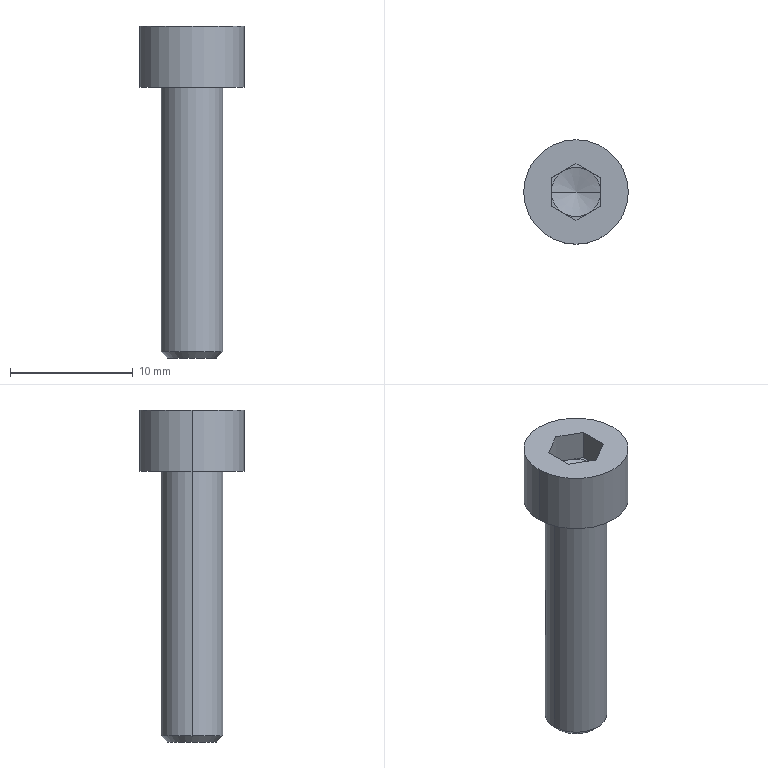Part | STEP file | TNSN20-Y20-F22-Part-10 | 1 solid | 23 faces | box 8.5 x 8.5 x 27 mm | volume 677.042 mm3 | plane 15 | cylinder 4 | cone 4 | commonest cylinder face diameters 5 x2 8.5 x2
STEP:
#1=CARTESIAN_POINT('',(14035.495,13710.046,28.5));
#2=VERTEX_POINT('',#1);
#3=CARTESIAN_POINT('',(14043.995,13710.046,28.5));
#4=VERTEX_POINT('',#3);
#5=CARTESIAN_POINT('',(14039.745,13710.046,28.5));
#6=DIRECTION('',(0.,0.,-1.));
#7=DIRECTION('',(1.,0.,0.));
#8=AXIS2_PLACEMENT_3D('',#5,#6,#7);
#9=CIRCLE('',#8,4.25);
#10=EDGE_CURVE('',#2,#4,#9,.T.);
#11=ORIENTED_EDGE('',*,*,#10,.F.);
#12=CARTESIAN_POINT('',(14039.745,13710.046,28.5));
#13=DIRECTION('',(0.,0.,-1.));
#14=DIRECTION('',(1.,0.,0.));
#15=AXIS2_PLACEMENT_3D('',#12,#13,#14);
#16=CIRCLE('',#15,4.25);
#17=EDGE_CURVE('',#4,#2,#16,.T.);
#18=ORIENTED_EDGE('',*,*,#17,.F.);
#19=EDGE_LOOP('',(#11,#18));
#20=FACE_OUTER_BOUND('',#19,.T.);
#21=CARTESIAN_POINT('',(14039.745,13712.356,28.5));
#22=VERTEX_POINT('',#21);
#23=CARTESIAN_POINT('',(14041.745,13711.201,28.5));
#24=VERTEX_POINT('',#23);
#25=CARTESIAN_POINT('',(14039.745,13712.356,28.5));
#26=DIRECTION('',(0.866,-0.5,0.));
#27=VECTOR('',#26,1000.);
#28=LINE('',#25,#27);
#29=EDGE_CURVE('',#22,#24,#28,.T.);
#30=ORIENTED_EDGE('',*,*,#29,.T.);
#31=CARTESIAN_POINT('',(14041.745,13708.892,28.5));
#32=VERTEX_POINT('',#31);
#33=CARTESIAN_POINT('',(14041.745,13711.201,28.5));
#34=DIRECTION('',(0.,-1.,0.));
#35=VECTOR('',#34,1000.);
#36=LINE('',#33,#35);
#37=EDGE_CURVE('',#24,#32,#36,.T.);
#38=ORIENTED_EDGE('',*,*,#37,.T.);
#39=CARTESIAN_POINT('',(14039.745,13707.737,28.5));
#40=VERTEX_POINT('',#39);
#41=CARTESIAN_POINT('',(14041.745,13708.892,28.5));
#42=DIRECTION('',(-0.866,-0.5,0.));
#43=VECTOR('',#42,1000.);
#44=LINE('',#41,#43);
#45=EDGE_CURVE('',#32,#40,#44,.T.);
#46=ORIENTED_EDGE('',*,*,#45,.T.);
#47=CARTESIAN_POINT('',(14037.745,13708.892,28.5));
#48=VERTEX_POINT('',#47);
#49=CARTESIAN_POINT('',(14039.745,13707.737,28.5));
#50=DIRECTION('',(-0.866,0.5,0.));
#51=VECTOR('',#50,1000.);
#52=LINE('',#49,#51);
#53=EDGE_CURVE('',#40,#48,#52,.T.);
#54=ORIENTED_EDGE('',*,*,#53,.T.);
#55=CARTESIAN_POINT('',(14037.745,13711.201,28.5));
#56=VERTEX_POINT('',#55);
#57=CARTESIAN_POINT('',(14037.745,13708.892,28.5));
#58=DIRECTION('',(0.,1.,0.));
#59=VECTOR('',#58,1000.);
#60=LINE('',#57,#59);
#61=EDGE_CURVE('',#48,#56,#60,.T.);
#62=ORIENTED_EDGE('',*,*,#61,.T.);
#63=CARTESIAN_POINT('',(14037.745,13711.201,28.5));
#64=DIRECTION('',(0.866,0.5,0.));
#65=VECTOR('',#64,1000.);
#66=LINE('',#63,#65);
#67=EDGE_CURVE('',#56,#22,#66,.T.);
#68=ORIENTED_EDGE('',*,*,#67,.T.);
#69=EDGE_LOOP('',(#30,#38,#46,#54,#62,#68));
#70=FACE_BOUND('',#69,.T.);
#71=CARTESIAN_POINT('',(14023.013,13724.653,28.5));
#72=DIRECTION('',(0.,0.,-1.));
#73=DIRECTION('',(1.,0.,0.));
#74=AXIS2_PLACEMENT_3D('',#71,#72,#73);
#75=PLANE('',#74);
#76=ADVANCED_FACE('',(#20,#70),#75,.F.);
#77=CARTESIAN_POINT('',(14043.995,13710.046,23.5));
#78=VERTEX_POINT('',#77);
#79=CARTESIAN_POINT('',(14035.495,13710.046,23.5));
#80=VERTEX_POINT('',#79);
#81=CARTESIAN_POINT('',(14039.745,13710.046,23.5));
#82=DIRECTION('',(0.,0.,-1.));
#83=DIRECTION('',(1.,0.,0.));
#84=AXIS2_PLACEMENT_3D('',#81,#82,#83);
#85=CIRCLE('',#84,4.25);
#86=EDGE_CURVE('',#78,#80,#85,.T.);
#87=ORIENTED_EDGE('',*,*,#86,.T.);
#88=CARTESIAN_POINT('',(14039.745,13710.046,23.5));
#89=DIRECTION('',(0.,0.,-1.));
#90=DIRECTION('',(1.,0.,0.));
#91=AXIS2_PLACEMENT_3D('',#88,#89,#90);
#92=CIRCLE('',#91,4.25);
#93=EDGE_CURVE('',#80,#78,#92,.T.);
#94=ORIENTED_EDGE('',*,*,#93,.T.);
#95=EDGE_LOOP('',(#87,#94));
#96=FACE_OUTER_BOUND('',#95,.T.);
#97=CARTESIAN_POINT('',(14037.245,13710.046,23.5));
#98=VERTEX_POINT('',#97);
#99=CARTESIAN_POINT('',(14042.245,13710.046,23.5));
#100=VERTEX_POINT('',#99);
#101=CARTESIAN_POINT('',(14039.745,13710.046,23.5));
#102=DIRECTION('',(0.,0.,-1.));
#103=DIRECTION('',(1.,0.,0.));
#104=AXIS2_PLACEMENT_3D('',#101,#102,#103);
#105=CIRCLE('',#104,2.5);
#106=EDGE_CURVE('',#98,#100,#105,.T.);
#107=ORIENTED_EDGE('',*,*,#106,.F.);
#108=CARTESIAN_POINT('',(14039.745,13710.046,23.5));
#109=DIRECTION('',(0.,0.,-1.));
#110=DIRECTION('',(1.,0.,0.));
#111=AXIS2_PLACEMENT_3D('',#108,#109,#110);
#112=CIRCLE('',#111,2.5);
#113=EDGE_CURVE('',#100,#98,#112,.T.);
#114=ORIENTED_EDGE('',*,*,#113,.F.);
#115=EDGE_LOOP('',(#107,#114));
#116=FACE_BOUND('',#115,.T.);
#117=CARTESIAN_POINT('',(14052.227,13724.653,23.5));
#118=DIRECTION('',(0.,0.,1.));
#119=DIRECTION('',(-1.,0.,0.));
#120=AXIS2_PLACEMENT_3D('',#117,#118,#119);
#121=PLANE('',#120);
#122=ADVANCED_FACE('',(#96,#116),#121,.F.);
#123=CARTESIAN_POINT('',(14041.754,13710.046,1.5));
#124=VERTEX_POINT('',#123);
#125=CARTESIAN_POINT('',(14037.735,13710.046,1.5));
#126=VERTEX_POINT('',#125);
#127=CARTESIAN_POINT('',(14039.745,13710.046,1.5));
#128=DIRECTION('',(0.,0.,-1.));
#129=DIRECTION('',(1.,0.,0.));
#130=AXIS2_PLACEMENT_3D('',#127,#128,#129);
#131=CIRCLE('',#130,2.009);
#132=EDGE_CURVE('',#124,#126,#131,.T.);
#133=ORIENTED_EDGE('',*,*,#132,.T.);
#134=CARTESIAN_POINT('',(14039.745,13710.046,1.5));
#135=DIRECTION('',(0.,0.,-1.));
#136=DIRECTION('',(1.,0.,0.));
#137=AXIS2_PLACEMENT_3D('',#134,#135,#136);
#138=CIRCLE('',#137,2.009);
#139=EDGE_CURVE('',#126,#124,#138,.T.);
#140=ORIENTED_EDGE('',*,*,#139,.T.);
#141=EDGE_LOOP('',(#133,#140));
#142=FACE_OUTER_BOUND('',#141,.T.);
#143=CARTESIAN_POINT('',(14045.647,13716.953,1.5));
#144=DIRECTION('',(0.,0.,1.));
#145=DIRECTION('',(-1.,0.,0.));
#146=AXIS2_PLACEMENT_3D('',#143,#144,#145);
#147=PLANE('',#146);
#148=ADVANCED_FACE('',(#142),#147,.F.);
#149=ORIENTED_EDGE('',*,*,#61,.F.);
#150=CARTESIAN_POINT('',(14037.745,13708.892,26.));
#151=VERTEX_POINT('',#150);
#152=CARTESIAN_POINT('',(14037.745,13708.892,26.));
#153=DIRECTION('',(0.,0.,1.));
#154=VECTOR('',#153,1000.);
#155=LINE('',#152,#154);
#156=EDGE_CURVE('',#151,#48,#155,.T.);
#157=ORIENTED_EDGE('',*,*,#156,.F.);
#158=CARTESIAN_POINT('',(14037.745,13710.046,26.));
#159=VERTEX_POINT('',#158);
#160=CARTESIAN_POINT('',(14037.745,13708.892,26.));
#161=DIRECTION('',(0.,1.,0.));
#162=VECTOR('',#161,1000.);
#163=LINE('',#160,#162);
#164=EDGE_CURVE('',#151,#159,#163,.T.);
#165=ORIENTED_EDGE('',*,*,#164,.T.);
#166=CARTESIAN_POINT('',(14037.745,13711.201,26.));
#167=VERTEX_POINT('',#166);
#168=CARTESIAN_POINT('',(14037.745,13710.046,26.));
#169=DIRECTION('',(0.,1.,0.));
#170=VECTOR('',#169,1000.);
#171=LINE('',#168,#170);
#172=EDGE_CURVE('',#159,#167,#171,.T.);
#173=ORIENTED_EDGE('',*,*,#172,.T.);
#174=CARTESIAN_POINT('',(14037.745,13711.201,26.));
#175=DIRECTION('',(0.,0.,1.));
#176=VECTOR('',#175,1000.);
#177=LINE('',#174,#176);
#178=EDGE_CURVE('',#167,#56,#177,.T.);
#179=ORIENTED_EDGE('',*,*,#178,.T.);
#180=EDGE_LOOP('',(#149,#157,#165,#173,#179));
#181=FACE_OUTER_BOUND('',#180,.T.);
#182=CARTESIAN_POINT('',(14037.745,13712.599,24.697));
#183=DIRECTION('',(1.,0.,0.));
#184=DIRECTION('',(0.,0.,1.));
#185=AXIS2_PLACEMENT_3D('',#182,#183,#184);
#186=PLANE('',#185);
#187=ADVANCED_FACE('',(#181),#186,.T.);
#188=ORIENTED_EDGE('',*,*,#67,.F.);
#189=ORIENTED_EDGE('',*,*,#178,.F.);
#190=CARTESIAN_POINT('',(14038.745,13711.778,26.));
#191=VERTEX_POINT('',#190);
#192=CARTESIAN_POINT('',(14037.745,13711.201,26.));
#193=DIRECTION('',(0.866,0.5,0.));
#194=VECTOR('',#193,1000.);
#195=LINE('',#192,#194);
#196=EDGE_CURVE('',#167,#191,#195,.T.);
#197=ORIENTED_EDGE('',*,*,#196,.T.);
#198=CARTESIAN_POINT('',(14039.745,13712.356,26.));
#199=VERTEX_POINT('',#198);
#200=CARTESIAN_POINT('',(14038.745,13711.778,26.));
#201=DIRECTION('',(0.866,0.5,0.));
#202=VECTOR('',#201,1000.);
#203=LINE('',#200,#202);
#204=EDGE_CURVE('',#191,#199,#203,.T.);
#205=ORIENTED_EDGE('',*,*,#204,.T.);
#206=CARTESIAN_POINT('',(14039.745,13712.356,26.));
#207=DIRECTION('',(0.,0.,1.));
#208=VECTOR('',#207,1000.);
#209=LINE('',#206,#208);
#210=EDGE_CURVE('',#199,#22,#209,.T.);
#211=ORIENTED_EDGE('',*,*,#210,.T.);
#212=EDGE_LOOP('',(#188,#189,#197,#205,#211));
#213=FACE_OUTER_BOUND('',#212,.T.);
#214=CARTESIAN_POINT('',(14040.956,13713.055,29.803));
#215=DIRECTION('',(0.5,-0.866,0.));
#216=DIRECTION('',(-0.866,-0.5,0.));
#217=AXIS2_PLACEMENT_3D('',#214,#215,#216);
#218=PLANE('',#217);
#219=ADVANCED_FACE('',(#213),#218,.T.);
#220=ORIENTED_EDGE('',*,*,#29,.F.);
#221=ORIENTED_EDGE('',*,*,#210,.F.);
#222=CARTESIAN_POINT('',(14040.745,13711.778,26.));
#223=VERTEX_POINT('',#222);
#224=CARTESIAN_POINT('',(14039.745,13712.356,26.));
#225=DIRECTION('',(0.866,-0.5,0.));
#226=VECTOR('',#225,1000.);
#227=LINE('',#224,#226);
#228=EDGE_CURVE('',#199,#223,#227,.T.);
#229=ORIENTED_EDGE('',*,*,#228,.T.);
#230=CARTESIAN_POINT('',(14041.745,13711.201,26.));
#231=VERTEX_POINT('',#230);
#232=CARTESIAN_POINT('',(14040.745,13711.778,26.));
#233=DIRECTION('',(0.866,-0.5,0.));
#234=VECTOR('',#233,1000.);
#235=LINE('',#232,#234);
#236=EDGE_CURVE('',#223,#231,#235,.T.);
#237=ORIENTED_EDGE('',*,*,#236,.T.);
#238=CARTESIAN_POINT('',(14041.745,13711.201,26.));
#239=DIRECTION('',(0.,0.,1.));
#240=VECTOR('',#239,1000.);
#241=LINE('',#238,#240);
#242=EDGE_CURVE('',#231,#24,#241,.T.);
#243=ORIENTED_EDGE('',*,*,#242,.T.);
#244=EDGE_LOOP('',(#220,#221,#229,#237,#243));
#245=FACE_OUTER_BOUND('',#244,.T.);
#246=CARTESIAN_POINT('',(14042.956,13710.502,29.803));
#247=DIRECTION('',(-0.5,-0.866,0.));
#248=DIRECTION('',(-0.866,0.5,0.));
#249=AXIS2_PLACEMENT_3D('',#246,#247,#248);
#250=PLANE('',#249);
#251=ADVANCED_FACE('',(#245),#250,.T.);
#252=ORIENTED_EDGE('',*,*,#37,.F.);
#253=ORIENTED_EDGE('',*,*,#242,.F.);
#254=CARTESIAN_POINT('',(14041.745,13710.046,26.));
#255=VERTEX_POINT('',#254);
#256=CARTESIAN_POINT('',(14041.745,13711.201,26.));
#257=DIRECTION('',(0.,-1.,0.));
#258=VECTOR('',#257,1000.);
#259=LINE('',#256,#258);
#260=EDGE_CURVE('',#231,#255,#259,.T.);
#261=ORIENTED_EDGE('',*,*,#260,.T.);
#262=CARTESIAN_POINT('',(14041.745,13708.892,26.));
#263=VERTEX_POINT('',#262);
#264=CARTESIAN_POINT('',(14041.745,13710.046,26.));
#265=DIRECTION('',(0.,-1.,0.));
#266=VECTOR('',#265,1000.);
#267=LINE('',#264,#266);
#268=EDGE_CURVE('',#255,#263,#267,.T.);
#269=ORIENTED_EDGE('',*,*,#268,.T.);
#270=CARTESIAN_POINT('',(14041.745,13708.892,26.));
#271=DIRECTION('',(0.,0.,1.));
#272=VECTOR('',#271,1000.);
#273=LINE('',#270,#272);
#274=EDGE_CURVE('',#263,#32,#273,.T.);
#275=ORIENTED_EDGE('',*,*,#274,.T.);
#276=EDGE_LOOP('',(#252,#253,#261,#269,#275));
#277=FACE_OUTER_BOUND('',#276,.T.);
#278=CARTESIAN_POINT('',(14041.745,13712.599,29.803));
#279=DIRECTION('',(-1.,0.,0.));
#280=DIRECTION('',(0.,0.,-1.));
#281=AXIS2_PLACEMENT_3D('',#278,#279,#280);
#282=PLANE('',#281);
#283=ADVANCED_FACE('',(#277),#282,.T.);
#284=ORIENTED_EDGE('',*,*,#45,.F.);
#285=ORIENTED_EDGE('',*,*,#274,.F.);
#286=CARTESIAN_POINT('',(14040.745,13708.314,26.));
#287=VERTEX_POINT('',#286);
#288=CARTESIAN_POINT('',(14041.745,13708.892,26.));
#289=DIRECTION('',(-0.866,-0.5,0.));
#290=VECTOR('',#289,1000.);
#291=LINE('',#288,#290);
#292=EDGE_CURVE('',#263,#287,#291,.T.);
#293=ORIENTED_EDGE('',*,*,#292,.T.);
#294=CARTESIAN_POINT('',(14039.745,13707.737,26.));
#295=VERTEX_POINT('',#294);
#296=CARTESIAN_POINT('',(14040.745,13708.314,26.));
#297=DIRECTION('',(-0.866,-0.5,0.));
#298=VECTOR('',#297,1000.);
#299=LINE('',#296,#298);
#300=EDGE_CURVE('',#287,#295,#299,.T.);
#301=ORIENTED_EDGE('',*,*,#300,.T.);
#302=CARTESIAN_POINT('',(14039.745,13707.737,26.));
#303=DIRECTION('',(0.,0.,1.));
#304=VECTOR('',#303,1000.);
#305=LINE('',#302,#304);
#306=EDGE_CURVE('',#295,#40,#305,.T.);
#307=ORIENTED_EDGE('',*,*,#306,.T.);
#308=EDGE_LOOP('',(#284,#285,#293,#301,#307));
#309=FACE_OUTER_BOUND('',#308,.T.);
#310=CARTESIAN_POINT('',(14038.534,13707.038,29.803));
#311=DIRECTION('',(-0.5,0.866,0.));
#312=DIRECTION('',(0.866,0.5,0.));
#313=AXIS2_PLACEMENT_3D('',#310,#311,#312);
#314=PLANE('',#313);
#315=ADVANCED_FACE('',(#309),#314,.T.);
#316=ORIENTED_EDGE('',*,*,#53,.F.);
#317=ORIENTED_EDGE('',*,*,#306,.F.);
#318=CARTESIAN_POINT('',(14038.745,13708.314,26.));
#319=VERTEX_POINT('',#318);
#320=CARTESIAN_POINT('',(14039.745,13707.737,26.));
#321=DIRECTION('',(-0.866,0.5,0.));
#322=VECTOR('',#321,1000.);
#323=LINE('',#320,#322);
#324=EDGE_CURVE('',#295,#319,#323,.T.);
#325=ORIENTED_EDGE('',*,*,#324,.T.);
#326=CARTESIAN_POINT('',(14038.745,13708.314,26.));
#327=DIRECTION('',(-0.866,0.5,0.));
#328=VECTOR('',#327,1000.);
#329=LINE('',#326,#328);
#330=EDGE_CURVE('',#319,#151,#329,.T.);
#331=ORIENTED_EDGE('',*,*,#330,.T.);
#332=ORIENTED_EDGE('',*,*,#156,.T.);
#333=EDGE_LOOP('',(#316,#317,#325,#331,#332));
#334=FACE_OUTER_BOUND('',#333,.T.);
#335=CARTESIAN_POINT('',(14036.534,13709.591,29.803));
#336=DIRECTION('',(0.5,0.866,0.));
#337=DIRECTION('',(0.866,-0.5,0.));
#338=AXIS2_PLACEMENT_3D('',#335,#336,#337);
#339=PLANE('',#338);
#340=ADVANCED_FACE('',(#334),#339,.T.);
#341=CARTESIAN_POINT('',(14039.745,13710.046,26.));
#342=DIRECTION('',(0.,0.,-1.));
#343=DIRECTION('',(1.,0.,0.));
#344=AXIS2_PLACEMENT_3D('',#341,#342,#343);
#345=CIRCLE('',#344,2.);
#346=EDGE_CURVE('',#255,#287,#345,.T.);
#347=ORIENTED_EDGE('',*,*,#346,.T.);
#348=ORIENTED_EDGE('',*,*,#292,.F.);
#349=ORIENTED_EDGE('',*,*,#268,.F.);
#350=EDGE_LOOP('',(#347,#348,#349));
#351=FACE_OUTER_BOUND('',#350,.T.);
#352=CARTESIAN_POINT('',(14039.745,13710.68,26.));
#353=DIRECTION('',(0.,0.,-1.));
#354=DIRECTION('',(1.,0.,0.));
#355=AXIS2_PLACEMENT_3D('',#352,#353,#354);
#356=PLANE('',#355);
#357=ADVANCED_FACE('',(#351),#356,.F.);
#358=ORIENTED_EDGE('',*,*,#300,.F.);
#359=CARTESIAN_POINT('',(14039.745,13710.046,26.));
#360=DIRECTION('',(0.,0.,-1.));
#361=DIRECTION('',(0.5,-0.866,0.));
#362=AXIS2_PLACEMENT_3D('',#359,#360,#361);
#363=CIRCLE('',#362,2.);
#364=EDGE_CURVE('',#287,#319,#363,.T.);
#365=ORIENTED_EDGE('',*,*,#364,.T.);
#366=ORIENTED_EDGE('',*,*,#324,.F.);
#367=EDGE_LOOP('',(#358,#365,#366));
#368=FACE_OUTER_BOUND('',#367,.T.);
#369=CARTESIAN_POINT('',(14038.184,13709.587,26.));
#370=DIRECTION('',(0.,0.,-1.));
#371=DIRECTION('',(1.,0.,0.));
#372=AXIS2_PLACEMENT_3D('',#369,#370,#371);
#373=PLANE('',#372);
#374=ADVANCED_FACE('',(#368),#373,.F.);
#375=CARTESIAN_POINT('',(14039.745,13710.046,26.));
#376=DIRECTION('',(0.,0.,-1.));
#377=DIRECTION('',(-0.5,-0.866,0.));
#378=AXIS2_PLACEMENT_3D('',#375,#376,#377);
#379=CIRCLE('',#378,2.);
#380=EDGE_CURVE('',#319,#159,#379,.T.);
#381=ORIENTED_EDGE('',*,*,#380,.T.);
#382=ORIENTED_EDGE('',*,*,#164,.F.);
#383=ORIENTED_EDGE('',*,*,#330,.F.);
#384=EDGE_LOOP('',(#381,#382,#383));
#385=FACE_OUTER_BOUND('',#384,.T.);
#386=CARTESIAN_POINT('',(14036.745,13710.68,26.));
#387=DIRECTION('',(0.,0.,-1.));
#388=DIRECTION('',(1.,0.,0.));
#389=AXIS2_PLACEMENT_3D('',#386,#387,#388);
#390=PLANE('',#389);
#391=ADVANCED_FACE('',(#385),#390,.F.);
#392=CARTESIAN_POINT('',(14039.745,13710.046,26.));
#393=DIRECTION('',(0.,0.,-1.));
#394=DIRECTION('',(-1.,0.,0.));
#395=AXIS2_PLACEMENT_3D('',#392,#393,#394);
#396=CIRCLE('',#395,2.);
#397=EDGE_CURVE('',#159,#191,#396,.T.);
#398=ORIENTED_EDGE('',*,*,#397,.T.);
#399=ORIENTED_EDGE('',*,*,#196,.F.);
#400=ORIENTED_EDGE('',*,*,#172,.F.);
#401=EDGE_LOOP('',(#398,#399,#400));
#402=FACE_OUTER_BOUND('',#401,.T.);
#403=CARTESIAN_POINT('',(14036.745,13712.412,26.));
#404=DIRECTION('',(0.,0.,-1.));
#405=DIRECTION('',(1.,0.,0.));
#406=AXIS2_PLACEMENT_3D('',#403,#404,#405);
#407=PLANE('',#406);
#408=ADVANCED_FACE('',(#402),#407,.F.);
#409=CARTESIAN_POINT('',(14039.745,13710.046,26.));
#410=DIRECTION('',(0.,0.,-1.));
#411=DIRECTION('',(-0.5,0.866,0.));
#412=AXIS2_PLACEMENT_3D('',#409,#410,#411);
#413=CIRCLE('',#412,2.);
#414=EDGE_CURVE('',#191,#223,#413,.T.);
#415=ORIENTED_EDGE('',*,*,#414,.T.);
#416=ORIENTED_EDGE('',*,*,#228,.F.);
#417=ORIENTED_EDGE('',*,*,#204,.F.);
#418=EDGE_LOOP('',(#415,#416,#417));
#419=FACE_OUTER_BOUND('',#418,.T.);
#420=CARTESIAN_POINT('',(14038.184,13713.628,26.));
#421=DIRECTION('',(0.,0.,-1.));
#422=DIRECTION('',(1.,0.,0.));
#423=AXIS2_PLACEMENT_3D('',#420,#421,#422);
#424=PLANE('',#423);
#425=ADVANCED_FACE('',(#419),#424,.F.);
#426=CARTESIAN_POINT('',(14039.745,13710.046,26.));
#427=DIRECTION('',(0.,0.,-1.));
#428=DIRECTION('',(0.5,0.866,0.));
#429=AXIS2_PLACEMENT_3D('',#426,#427,#428);
#430=CIRCLE('',#429,2.);
#431=EDGE_CURVE('',#223,#255,#430,.T.);
#432=ORIENTED_EDGE('',*,*,#431,.T.);
#433=ORIENTED_EDGE('',*,*,#260,.F.);
#434=ORIENTED_EDGE('',*,*,#236,.F.);
#435=EDGE_LOOP('',(#432,#433,#434));
#436=FACE_OUTER_BOUND('',#435,.T.);
#437=CARTESIAN_POINT('',(14039.745,13712.412,26.));
#438=DIRECTION('',(0.,0.,-1.));
#439=DIRECTION('',(1.,0.,0.));
#440=AXIS2_PLACEMENT_3D('',#437,#438,#439);
#441=PLANE('',#440);
#442=ADVANCED_FACE('',(#436),#441,.F.);
#443=ORIENTED_EDGE('',*,*,#93,.F.);
#444=CARTESIAN_POINT('',(14035.495,13710.046,28.5));
#445=DIRECTION('',(0.,0.,-1.));
#446=VECTOR('',#445,1000.);
#447=LINE('',#444,#446);
#448=EDGE_CURVE('',#2,#80,#447,.T.);
#449=ORIENTED_EDGE('',*,*,#448,.F.);
#450=ORIENTED_EDGE('',*,*,#10,.T.);
#451=CARTESIAN_POINT('',(14043.995,13710.046,28.5));
#452=DIRECTION('',(0.,0.,-1.));
#453=VECTOR('',#452,1000.);
#454=LINE('',#451,#453);
#455=EDGE_CURVE('',#4,#78,#454,.T.);
#456=ORIENTED_EDGE('',*,*,#455,.T.);
#457=EDGE_LOOP('',(#443,#449,#450,#456));
#458=FACE_OUTER_BOUND('',#457,.T.);
#459=CARTESIAN_POINT('',(14039.745,13710.046,26.));
#460=DIRECTION('',(0.,0.,-1.));
#461=DIRECTION('',(-1.,0.,0.));
#462=AXIS2_PLACEMENT_3D('',#459,#460,#461);
#463=CYLINDRICAL_SURFACE('',#462,4.25);
#464=ADVANCED_FACE('',(#458),#463,.T.);
#465=ORIENTED_EDGE('',*,*,#17,.T.);
#466=ORIENTED_EDGE('',*,*,#448,.T.);
#467=ORIENTED_EDGE('',*,*,#86,.F.);
#468=ORIENTED_EDGE('',*,*,#455,.F.);
#469=EDGE_LOOP('',(#465,#466,#467,#468));
#470=FACE_OUTER_BOUND('',#469,.T.);
#471=CARTESIAN_POINT('',(14039.745,13710.046,26.));
#472=DIRECTION('',(0.,0.,-1.));
#473=DIRECTION('',(-1.,0.,0.));
#474=AXIS2_PLACEMENT_3D('',#471,#472,#473);
#475=CYLINDRICAL_SURFACE('',#474,4.25);
#476=ADVANCED_FACE('',(#470),#475,.T.);
#477=CARTESIAN_POINT('',(14037.245,13710.046,1.99));
#478=VERTEX_POINT('',#477);
#479=CARTESIAN_POINT('',(14042.245,13710.046,1.99));
#480=VERTEX_POINT('',#479);
#481=CARTESIAN_POINT('',(14039.745,13710.046,1.99));
#482=DIRECTION('',(0.,0.,-1.));
#483=DIRECTION('',(1.,0.,0.));
#484=AXIS2_PLACEMENT_3D('',#481,#482,#483);
#485=CIRCLE('',#484,2.5);
#486=EDGE_CURVE('',#478,#480,#485,.T.);
#487=ORIENTED_EDGE('',*,*,#486,.F.);
#488=CARTESIAN_POINT('',(14037.245,13710.046,23.5));
#489=DIRECTION('',(0.,0.,-1.));
#490=VECTOR('',#489,1000.);
#491=LINE('',#488,#490);
#492=EDGE_CURVE('',#98,#478,#491,.T.);
#493=ORIENTED_EDGE('',*,*,#492,.F.);
#494=ORIENTED_EDGE('',*,*,#106,.T.);
#495=CARTESIAN_POINT('',(14042.245,13710.046,23.5));
#496=DIRECTION('',(0.,0.,-1.));
#497=VECTOR('',#496,1000.);
#498=LINE('',#495,#497);
#499=EDGE_CURVE('',#100,#480,#498,.T.);
#500=ORIENTED_EDGE('',*,*,#499,.T.);
#501=EDGE_LOOP('',(#487,#493,#494,#500));
#502=FACE_OUTER_BOUND('',#501,.T.);
#503=CARTESIAN_POINT('',(14039.745,13710.046,12.745));
#504=DIRECTION('',(0.,0.,-1.));
#505=DIRECTION('',(-1.,0.,0.));
#506=AXIS2_PLACEMENT_3D('',#503,#504,#505);
#507=CYLINDRICAL_SURFACE('',#506,2.5);
#508=ADVANCED_FACE('',(#502),#507,.T.);
#509=ORIENTED_EDGE('',*,*,#113,.T.);
#510=ORIENTED_EDGE('',*,*,#492,.T.);
#511=CARTESIAN_POINT('',(14039.745,13710.046,1.99));
#512=DIRECTION('',(0.,0.,-1.));
#513=DIRECTION('',(1.,0.,0.));
#514=AXIS2_PLACEMENT_3D('',#511,#512,#513);
#515=CIRCLE('',#514,2.5);
#516=EDGE_CURVE('',#480,#478,#515,.T.);
#517=ORIENTED_EDGE('',*,*,#516,.F.);
#518=ORIENTED_EDGE('',*,*,#499,.F.);
#519=EDGE_LOOP('',(#509,#510,#517,#518));
#520=FACE_OUTER_BOUND('',#519,.T.);
#521=CARTESIAN_POINT('',(14039.745,13710.046,12.745));
#522=DIRECTION('',(0.,0.,-1.));
#523=DIRECTION('',(-1.,0.,0.));
#524=AXIS2_PLACEMENT_3D('',#521,#522,#523);
#525=CYLINDRICAL_SURFACE('',#524,2.5);
#526=ADVANCED_FACE('',(#520),#525,.T.);
#527=ORIENTED_EDGE('',*,*,#139,.F.);
#528=CARTESIAN_POINT('',(14037.245,13710.046,1.99));
#529=DIRECTION('',(0.7071,0.,-0.7071));
#530=VECTOR('',#529,1000.);
#531=LINE('',#528,#530);
#532=EDGE_CURVE('',#478,#126,#531,.T.);
#533=ORIENTED_EDGE('',*,*,#532,.F.);
#534=ORIENTED_EDGE('',*,*,#486,.T.);
#535=CARTESIAN_POINT('',(14042.245,13710.046,1.99));
#536=DIRECTION('',(-0.7071,0.,-0.7071));
#537=VECTOR('',#536,1000.);
#538=LINE('',#535,#537);
#539=EDGE_CURVE('',#480,#124,#538,.T.);
#540=ORIENTED_EDGE('',*,*,#539,.T.);
#541=EDGE_LOOP('',(#527,#533,#534,#540));
#542=FACE_OUTER_BOUND('',#541,.T.);
#543=CARTESIAN_POINT('',(14039.745,13710.046,999.49));
#544=DIRECTION('',(0.,0.,1.));
#545=DIRECTION('',(-1.,0.,0.));
#546=AXIS2_PLACEMENT_3D('',#543,#544,#545);
#547=CONICAL_SURFACE('',#546,1000.,0.7854);
#548=ADVANCED_FACE('',(#542),#547,.T.);
#549=ORIENTED_EDGE('',*,*,#516,.T.);
#550=ORIENTED_EDGE('',*,*,#532,.T.);
#551=ORIENTED_EDGE('',*,*,#132,.F.);
#552=ORIENTED_EDGE('',*,*,#539,.F.);
#553=EDGE_LOOP('',(#549,#550,#551,#552));
#554=FACE_OUTER_BOUND('',#553,.T.);
#555=CARTESIAN_POINT('',(14039.745,13710.046,999.49));
#556=DIRECTION('',(0.,0.,1.));
#557=DIRECTION('',(-1.,0.,0.));
#558=AXIS2_PLACEMENT_3D('',#555,#556,#557);
#559=CONICAL_SURFACE('',#558,1000.,0.7854);
#560=ADVANCED_FACE('',(#554),#559,.T.);
#561=ORIENTED_EDGE('',*,*,#431,.F.);
#562=ORIENTED_EDGE('',*,*,#414,.F.);
#563=ORIENTED_EDGE('',*,*,#397,.F.);
#564=CARTESIAN_POINT('',(14039.745,13710.046,25.464));
#565=VERTEX_POINT('',#564);
#566=CARTESIAN_POINT('',(14037.745,13710.046,26.));
#567=DIRECTION('',(0.9659,0.,-0.2588));
#568=VECTOR('',#567,1000.);
#569=LINE('',#566,#568);
#570=EDGE_CURVE('',#159,#565,#569,.T.);
#571=ORIENTED_EDGE('',*,*,#570,.T.);
#572=CARTESIAN_POINT('',(14041.745,13710.046,26.));
#573=DIRECTION('',(-0.9659,0.,-0.2588));
#574=VECTOR('',#573,1000.);
#575=LINE('',#572,#574);
#576=EDGE_CURVE('',#255,#565,#575,.T.);
#577=ORIENTED_EDGE('',*,*,#576,.F.);
#578=EDGE_LOOP('',(#561,#562,#563,#571,#577));
#579=FACE_OUTER_BOUND('',#578,.T.);
#580=CARTESIAN_POINT('',(14039.745,13710.046,1025.464));
#581=DIRECTION('',(0.,0.,1.));
#582=DIRECTION('',(-1.,0.,0.));
#583=AXIS2_PLACEMENT_3D('',#580,#581,#582);
#584=CONICAL_SURFACE('',#583,3732.051,1.309);
#585=ADVANCED_FACE('',(#579),#584,.F.);
#586=ORIENTED_EDGE('',*,*,#570,.F.);
#587=ORIENTED_EDGE('',*,*,#380,.F.);
#588=ORIENTED_EDGE('',*,*,#364,.F.);
#589=ORIENTED_EDGE('',*,*,#346,.F.);
#590=ORIENTED_EDGE('',*,*,#576,.T.);
#591=EDGE_LOOP('',(#586,#587,#588,#589,#590));
#592=FACE_OUTER_BOUND('',#591,.T.);
#593=CARTESIAN_POINT('',(14039.745,13710.046,1025.464));
#594=DIRECTION('',(0.,0.,1.));
#595=DIRECTION('',(-1.,0.,0.));
#596=AXIS2_PLACEMENT_3D('',#593,#594,#595);
#597=CONICAL_SURFACE('',#596,3732.051,1.309);
#598=ADVANCED_FACE('',(#592),#597,.F.);
#599=CLOSED_SHELL('',(#76,#122,#148,#187,#219,#251,#283,#315,#340,#357,#374,#391,#408,#425,#442,#464,#476,#508,#526,#548,#560,#585,#598));
#600=MANIFOLD_SOLID_BREP('',#599);
#601=CARTESIAN_POINT('',(0.,0.,0.));
#602=DIRECTION('',(0.,0.,1.));
#603=DIRECTION('',(1.,0.,0.));
#604=AXIS2_PLACEMENT_3D('',#601,#602,#603);
#605=(LENGTH_UNIT()NAMED_UNIT(*)SI_UNIT(.MILLI.,.METRE.));
#606=UNCERTAINTY_MEASURE_WITH_UNIT(LENGTH_MEASURE(0.00001),#605,'','');
#607=(NAMED_UNIT(*)PLANE_ANGLE_UNIT()SI_UNIT($,.RADIAN.));
#608=(NAMED_UNIT(*)SI_UNIT($,.STERADIAN.)SOLID_ANGLE_UNIT());
#609=(GEOMETRIC_REPRESENTATION_CONTEXT(3)GLOBAL_UNCERTAINTY_ASSIGNED_CONTEXT((#606))GLOBAL_UNIT_ASSIGNED_CONTEXT((#605,#607,#608))REPRESENTATION_CONTEXT('',''));
#610=ADVANCED_BREP_SHAPE_REPRESENTATION('',(#600,#604),#609);